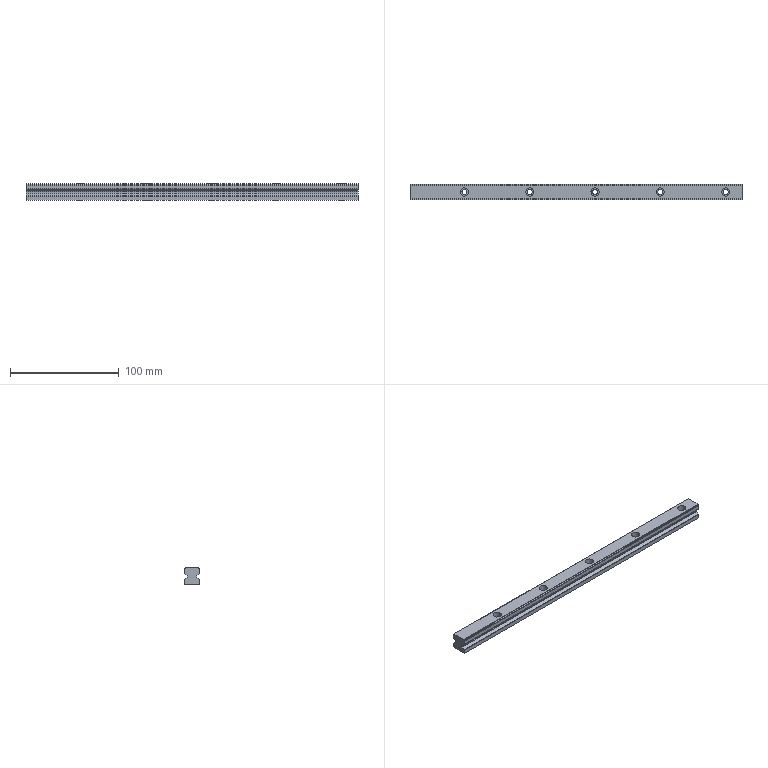Part | STEP file | Tube feed_id870_x_t | 1 solid | 45 faces | box 305 x 14.464 x 15 mm | volume 56339 mm3 | cylinder 26 | plane 19 | commonest cylinder face diameters 1 x9 0.6 x6 4.5 x5 7.5 x5 1.005 x1